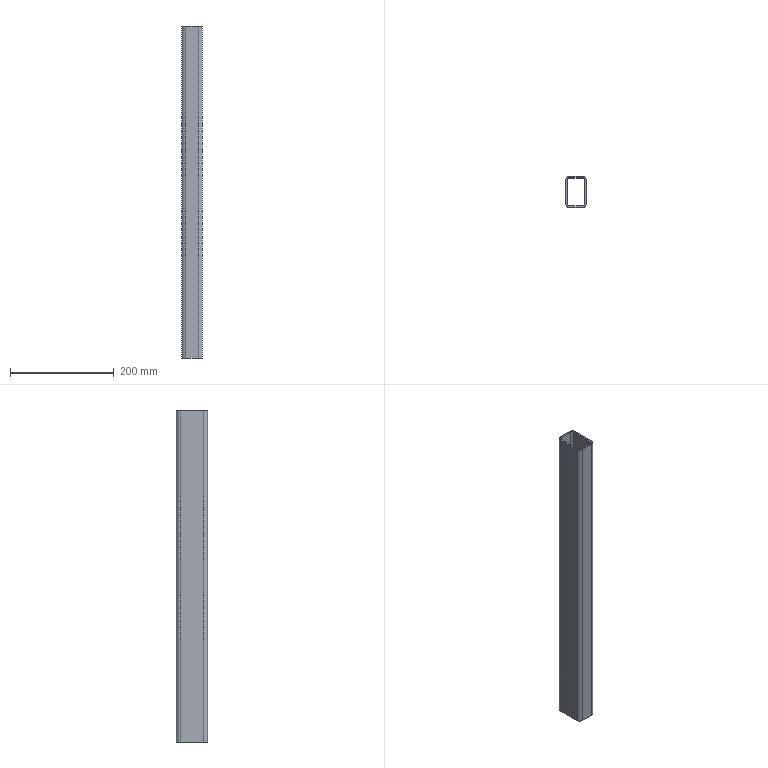Part | SolidWorks | features BaseBody 1 | 1 solid | 18 faces | box 40 x 60 x 640 mm | volume 341182 mm3 | plane 10 | cylinder 8 | commonest cylinder face diameters 9 x4 15 x4
STEP:
#1=CARTESIAN_POINT('',(17.,22.5,30.));
#2=VERTEX_POINT('',#1);
#3=CARTESIAN_POINT('',(17.,22.5,670.));
#4=VERTEX_POINT('',#3);
#5=CARTESIAN_POINT('',(17.,22.5,0.));
#6=DIRECTION('',(0.,0.,1.));
#7=VECTOR('',#6,1000.);
#8=LINE('',#5,#7);
#9=EDGE_CURVE('',#2,#4,#8,.T.);
#10=ORIENTED_EDGE('',*,*,#9,.F.);
#11=CARTESIAN_POINT('',(17.,-22.5,30.));
#12=VERTEX_POINT('',#11);
#13=CARTESIAN_POINT('',(17.,22.5,30.));
#14=DIRECTION('',(0.,1.,0.));
#15=VECTOR('',#14,1000.);
#16=LINE('',#13,#15);
#17=EDGE_CURVE('',#12,#2,#16,.T.);
#18=ORIENTED_EDGE('',*,*,#17,.F.);
#19=CARTESIAN_POINT('',(17.,-22.5,670.));
#20=VERTEX_POINT('',#19);
#21=CARTESIAN_POINT('',(17.,-22.5,0.));
#22=DIRECTION('',(0.,0.,-1.));
#23=VECTOR('',#22,1000.);
#24=LINE('',#21,#23);
#25=EDGE_CURVE('',#20,#12,#24,.T.);
#26=ORIENTED_EDGE('',*,*,#25,.F.);
#27=CARTESIAN_POINT('',(17.,22.5,670.));
#28=DIRECTION('',(0.,-1.,0.));
#29=VECTOR('',#28,1000.);
#30=LINE('',#27,#29);
#31=EDGE_CURVE('',#4,#20,#30,.T.);
#32=ORIENTED_EDGE('',*,*,#31,.F.);
#33=EDGE_LOOP('',(#10,#18,#26,#32));
#34=FACE_OUTER_BOUND('',#33,.T.);
#35=CARTESIAN_POINT('',(17.,22.5,0.));
#36=DIRECTION('',(1.,0.,0.));
#37=DIRECTION('',(0.,1.,0.));
#38=AXIS2_PLACEMENT_3D('',#35,#36,#37);
#39=PLANE('',#38);
#40=ADVANCED_FACE('',(#34),#39,.F.);
#41=CARTESIAN_POINT('',(-17.,-22.5,670.));
#42=VERTEX_POINT('',#41);
#43=CARTESIAN_POINT('',(-17.,22.5,670.));
#44=VERTEX_POINT('',#43);
#45=CARTESIAN_POINT('',(-17.,0.,670.));
#46=DIRECTION('',(0.,1.,0.));
#47=VECTOR('',#46,1000.);
#48=LINE('',#45,#47);
#49=EDGE_CURVE('',#42,#44,#48,.T.);
#50=ORIENTED_EDGE('',*,*,#49,.T.);
#51=CARTESIAN_POINT('',(-12.5,27.,670.));
#52=VERTEX_POINT('',#51);
#53=CARTESIAN_POINT('',(-12.5,22.5,670.));
#54=DIRECTION('',(0.,0.,-1.));
#55=DIRECTION('',(1.,0.,0.));
#56=AXIS2_PLACEMENT_3D('',#53,#54,#55);
#57=CIRCLE('',#56,4.5);
#58=EDGE_CURVE('',#44,#52,#57,.T.);
#59=ORIENTED_EDGE('',*,*,#58,.T.);
#60=CARTESIAN_POINT('',(12.5,27.,670.));
#61=VERTEX_POINT('',#60);
#62=CARTESIAN_POINT('',(0.,27.,670.));
#63=DIRECTION('',(1.,0.,0.));
#64=VECTOR('',#63,1000.);
#65=LINE('',#62,#64);
#66=EDGE_CURVE('',#52,#61,#65,.T.);
#67=ORIENTED_EDGE('',*,*,#66,.T.);
#68=CARTESIAN_POINT('',(12.5,22.5,670.));
#69=DIRECTION('',(0.,0.,-1.));
#70=DIRECTION('',(1.,0.,0.));
#71=AXIS2_PLACEMENT_3D('',#68,#69,#70);
#72=CIRCLE('',#71,4.5);
#73=EDGE_CURVE('',#61,#4,#72,.T.);
#74=ORIENTED_EDGE('',*,*,#73,.T.);
#75=ORIENTED_EDGE('',*,*,#31,.T.);
#76=CARTESIAN_POINT('',(12.5,-27.,670.));
#77=VERTEX_POINT('',#76);
#78=CARTESIAN_POINT('',(12.5,-22.5,670.));
#79=DIRECTION('',(0.,0.,-1.));
#80=DIRECTION('',(1.,0.,0.));
#81=AXIS2_PLACEMENT_3D('',#78,#79,#80);
#82=CIRCLE('',#81,4.5);
#83=EDGE_CURVE('',#20,#77,#82,.T.);
#84=ORIENTED_EDGE('',*,*,#83,.T.);
#85=CARTESIAN_POINT('',(-12.5,-27.,670.));
#86=VERTEX_POINT('',#85);
#87=CARTESIAN_POINT('',(0.,-27.,670.));
#88=DIRECTION('',(-1.,0.,0.));
#89=VECTOR('',#88,1000.);
#90=LINE('',#87,#89);
#91=EDGE_CURVE('',#77,#86,#90,.T.);
#92=ORIENTED_EDGE('',*,*,#91,.T.);
#93=CARTESIAN_POINT('',(-12.5,-22.5,670.));
#94=DIRECTION('',(0.,0.,-1.));
#95=DIRECTION('',(1.,0.,0.));
#96=AXIS2_PLACEMENT_3D('',#93,#94,#95);
#97=CIRCLE('',#96,4.5);
#98=EDGE_CURVE('',#86,#42,#97,.T.);
#99=ORIENTED_EDGE('',*,*,#98,.T.);
#100=EDGE_LOOP('',(#50,#59,#67,#74,#75,#84,#92,#99));
#101=FACE_BOUND('',#100,.T.);
#102=CARTESIAN_POINT('',(12.5,30.,670.));
#103=VERTEX_POINT('',#102);
#104=CARTESIAN_POINT('',(-12.5,30.,670.));
#105=VERTEX_POINT('',#104);
#106=CARTESIAN_POINT('',(0.,30.,670.));
#107=DIRECTION('',(-1.,0.,0.));
#108=VECTOR('',#107,1000.);
#109=LINE('',#106,#108);
#110=EDGE_CURVE('',#103,#105,#109,.T.);
#111=ORIENTED_EDGE('',*,*,#110,.T.);
#112=CARTESIAN_POINT('',(-20.,22.5,670.));
#113=VERTEX_POINT('',#112);
#114=CARTESIAN_POINT('',(-12.5,22.5,670.));
#115=DIRECTION('',(0.,0.,1.));
#116=DIRECTION('',(1.,0.,0.));
#117=AXIS2_PLACEMENT_3D('',#114,#115,#116);
#118=CIRCLE('',#117,7.5);
#119=EDGE_CURVE('',#105,#113,#118,.T.);
#120=ORIENTED_EDGE('',*,*,#119,.T.);
#121=CARTESIAN_POINT('',(-20.,-22.5,670.));
#122=VERTEX_POINT('',#121);
#123=CARTESIAN_POINT('',(-20.,0.,670.));
#124=DIRECTION('',(0.,-1.,0.));
#125=VECTOR('',#124,1000.);
#126=LINE('',#123,#125);
#127=EDGE_CURVE('',#113,#122,#126,.T.);
#128=ORIENTED_EDGE('',*,*,#127,.T.);
#129=CARTESIAN_POINT('',(-12.5,-30.,670.));
#130=VERTEX_POINT('',#129);
#131=CARTESIAN_POINT('',(-12.5,-22.5,670.));
#132=DIRECTION('',(0.,0.,1.));
#133=DIRECTION('',(1.,0.,0.));
#134=AXIS2_PLACEMENT_3D('',#131,#132,#133);
#135=CIRCLE('',#134,7.5);
#136=EDGE_CURVE('',#122,#130,#135,.T.);
#137=ORIENTED_EDGE('',*,*,#136,.T.);
#138=CARTESIAN_POINT('',(12.5,-30.,670.));
#139=VERTEX_POINT('',#138);
#140=CARTESIAN_POINT('',(0.,-30.,670.));
#141=DIRECTION('',(1.,0.,0.));
#142=VECTOR('',#141,1000.);
#143=LINE('',#140,#142);
#144=EDGE_CURVE('',#130,#139,#143,.T.);
#145=ORIENTED_EDGE('',*,*,#144,.T.);
#146=CARTESIAN_POINT('',(20.,-22.5,670.));
#147=VERTEX_POINT('',#146);
#148=CARTESIAN_POINT('',(12.5,-22.5,670.));
#149=DIRECTION('',(0.,0.,1.));
#150=DIRECTION('',(1.,0.,0.));
#151=AXIS2_PLACEMENT_3D('',#148,#149,#150);
#152=CIRCLE('',#151,7.5);
#153=EDGE_CURVE('',#139,#147,#152,.T.);
#154=ORIENTED_EDGE('',*,*,#153,.T.);
#155=CARTESIAN_POINT('',(20.,22.5,670.));
#156=VERTEX_POINT('',#155);
#157=CARTESIAN_POINT('',(20.,0.,670.));
#158=DIRECTION('',(0.,1.,0.));
#159=VECTOR('',#158,1000.);
#160=LINE('',#157,#159);
#161=EDGE_CURVE('',#147,#156,#160,.T.);
#162=ORIENTED_EDGE('',*,*,#161,.T.);
#163=CARTESIAN_POINT('',(12.5,22.5,670.));
#164=DIRECTION('',(0.,0.,1.));
#165=DIRECTION('',(1.,0.,0.));
#166=AXIS2_PLACEMENT_3D('',#163,#164,#165);
#167=CIRCLE('',#166,7.5);
#168=EDGE_CURVE('',#156,#103,#167,.T.);
#169=ORIENTED_EDGE('',*,*,#168,.T.);
#170=EDGE_LOOP('',(#111,#120,#128,#137,#145,#154,#162,#169));
#171=FACE_OUTER_BOUND('',#170,.T.);
#172=CARTESIAN_POINT('',(0.,0.,670.));
#173=DIRECTION('',(0.,0.,1.));
#174=DIRECTION('',(1.,0.,0.));
#175=AXIS2_PLACEMENT_3D('',#172,#173,#174);
#176=PLANE('',#175);
#177=ADVANCED_FACE('',(#101,#171),#176,.T.);
#178=CARTESIAN_POINT('',(12.5,27.,30.));
#179=VERTEX_POINT('',#178);
#180=CARTESIAN_POINT('',(12.5,27.,0.));
#181=DIRECTION('',(0.,0.,1.));
#182=VECTOR('',#181,1000.);
#183=LINE('',#180,#182);
#184=EDGE_CURVE('',#179,#61,#183,.T.);
#185=ORIENTED_EDGE('',*,*,#184,.F.);
#186=CARTESIAN_POINT('',(12.5,22.5,30.));
#187=DIRECTION('',(0.,0.,1.));
#188=DIRECTION('',(1.,0.,0.));
#189=AXIS2_PLACEMENT_3D('',#186,#187,#188);
#190=CIRCLE('',#189,4.5);
#191=EDGE_CURVE('',#2,#179,#190,.T.);
#192=ORIENTED_EDGE('',*,*,#191,.F.);
#193=ORIENTED_EDGE('',*,*,#9,.T.);
#194=ORIENTED_EDGE('',*,*,#73,.F.);
#195=EDGE_LOOP('',(#185,#192,#193,#194));
#196=FACE_OUTER_BOUND('',#195,.T.);
#197=CARTESIAN_POINT('',(12.5,22.5,0.));
#198=DIRECTION('',(0.,0.,1.));
#199=DIRECTION('',(1.,0.,0.));
#200=AXIS2_PLACEMENT_3D('',#197,#198,#199);
#201=CYLINDRICAL_SURFACE('',#200,4.5);
#202=ADVANCED_FACE('',(#196),#201,.F.);
#203=CARTESIAN_POINT('',(-17.,22.5,30.));
#204=VERTEX_POINT('',#203);
#205=CARTESIAN_POINT('',(-12.5,27.,30.));
#206=VERTEX_POINT('',#205);
#207=CARTESIAN_POINT('',(-12.5,22.5,30.));
#208=DIRECTION('',(0.,0.,-1.));
#209=DIRECTION('',(1.,0.,0.));
#210=AXIS2_PLACEMENT_3D('',#207,#208,#209);
#211=CIRCLE('',#210,4.5);
#212=EDGE_CURVE('',#204,#206,#211,.T.);
#213=ORIENTED_EDGE('',*,*,#212,.F.);
#214=CARTESIAN_POINT('',(-17.,-22.5,30.));
#215=VERTEX_POINT('',#214);
#216=CARTESIAN_POINT('',(-17.,0.,30.));
#217=DIRECTION('',(0.,1.,0.));
#218=VECTOR('',#217,1000.);
#219=LINE('',#216,#218);
#220=EDGE_CURVE('',#215,#204,#219,.T.);
#221=ORIENTED_EDGE('',*,*,#220,.F.);
#222=CARTESIAN_POINT('',(-12.5,-27.,30.));
#223=VERTEX_POINT('',#222);
#224=CARTESIAN_POINT('',(-12.5,-22.5,30.));
#225=DIRECTION('',(0.,0.,-1.));
#226=DIRECTION('',(1.,0.,0.));
#227=AXIS2_PLACEMENT_3D('',#224,#225,#226);
#228=CIRCLE('',#227,4.5);
#229=EDGE_CURVE('',#223,#215,#228,.T.);
#230=ORIENTED_EDGE('',*,*,#229,.F.);
#231=CARTESIAN_POINT('',(12.5,-27.,30.));
#232=VERTEX_POINT('',#231);
#233=CARTESIAN_POINT('',(0.,-27.,30.));
#234=DIRECTION('',(-1.,0.,0.));
#235=VECTOR('',#234,1000.);
#236=LINE('',#233,#235);
#237=EDGE_CURVE('',#232,#223,#236,.T.);
#238=ORIENTED_EDGE('',*,*,#237,.F.);
#239=CARTESIAN_POINT('',(12.5,-22.5,30.));
#240=DIRECTION('',(0.,0.,-1.));
#241=DIRECTION('',(1.,0.,0.));
#242=AXIS2_PLACEMENT_3D('',#239,#240,#241);
#243=CIRCLE('',#242,4.5);
#244=EDGE_CURVE('',#12,#232,#243,.T.);
#245=ORIENTED_EDGE('',*,*,#244,.F.);
#246=ORIENTED_EDGE('',*,*,#17,.T.);
#247=ORIENTED_EDGE('',*,*,#191,.T.);
#248=CARTESIAN_POINT('',(0.,27.,30.));
#249=DIRECTION('',(1.,0.,0.));
#250=VECTOR('',#249,1000.);
#251=LINE('',#248,#250);
#252=EDGE_CURVE('',#206,#179,#251,.T.);
#253=ORIENTED_EDGE('',*,*,#252,.F.);
#254=EDGE_LOOP('',(#213,#221,#230,#238,#245,#246,#247,#253));
#255=FACE_BOUND('',#254,.T.);
#256=CARTESIAN_POINT('',(-12.5,30.,30.));
#257=VERTEX_POINT('',#256);
#258=CARTESIAN_POINT('',(-20.,22.5,30.));
#259=VERTEX_POINT('',#258);
#260=CARTESIAN_POINT('',(-12.5,22.5,30.));
#261=DIRECTION('',(0.,0.,1.));
#262=DIRECTION('',(1.,0.,0.));
#263=AXIS2_PLACEMENT_3D('',#260,#261,#262);
#264=CIRCLE('',#263,7.5);
#265=EDGE_CURVE('',#257,#259,#264,.T.);
#266=ORIENTED_EDGE('',*,*,#265,.F.);
#267=CARTESIAN_POINT('',(12.5,30.,30.));
#268=VERTEX_POINT('',#267);
#269=CARTESIAN_POINT('',(0.,30.,30.));
#270=DIRECTION('',(-1.,0.,0.));
#271=VECTOR('',#270,1000.);
#272=LINE('',#269,#271);
#273=EDGE_CURVE('',#268,#257,#272,.T.);
#274=ORIENTED_EDGE('',*,*,#273,.F.);
#275=CARTESIAN_POINT('',(20.,22.5,30.));
#276=VERTEX_POINT('',#275);
#277=CARTESIAN_POINT('',(12.5,22.5,30.));
#278=DIRECTION('',(0.,0.,1.));
#279=DIRECTION('',(1.,0.,0.));
#280=AXIS2_PLACEMENT_3D('',#277,#278,#279);
#281=CIRCLE('',#280,7.5);
#282=EDGE_CURVE('',#276,#268,#281,.T.);
#283=ORIENTED_EDGE('',*,*,#282,.F.);
#284=CARTESIAN_POINT('',(20.,-22.5,30.));
#285=VERTEX_POINT('',#284);
#286=CARTESIAN_POINT('',(20.,0.,30.));
#287=DIRECTION('',(0.,1.,0.));
#288=VECTOR('',#287,1000.);
#289=LINE('',#286,#288);
#290=EDGE_CURVE('',#285,#276,#289,.T.);
#291=ORIENTED_EDGE('',*,*,#290,.F.);
#292=CARTESIAN_POINT('',(12.5,-30.,30.));
#293=VERTEX_POINT('',#292);
#294=CARTESIAN_POINT('',(12.5,-22.5,30.));
#295=DIRECTION('',(0.,0.,1.));
#296=DIRECTION('',(1.,0.,0.));
#297=AXIS2_PLACEMENT_3D('',#294,#295,#296);
#298=CIRCLE('',#297,7.5);
#299=EDGE_CURVE('',#293,#285,#298,.T.);
#300=ORIENTED_EDGE('',*,*,#299,.F.);
#301=CARTESIAN_POINT('',(-12.5,-30.,30.));
#302=VERTEX_POINT('',#301);
#303=CARTESIAN_POINT('',(0.,-30.,30.));
#304=DIRECTION('',(1.,0.,0.));
#305=VECTOR('',#304,1000.);
#306=LINE('',#303,#305);
#307=EDGE_CURVE('',#302,#293,#306,.T.);
#308=ORIENTED_EDGE('',*,*,#307,.F.);
#309=CARTESIAN_POINT('',(-20.,-22.5,30.));
#310=VERTEX_POINT('',#309);
#311=CARTESIAN_POINT('',(-12.5,-22.5,30.));
#312=DIRECTION('',(0.,0.,1.));
#313=DIRECTION('',(1.,0.,0.));
#314=AXIS2_PLACEMENT_3D('',#311,#312,#313);
#315=CIRCLE('',#314,7.5);
#316=EDGE_CURVE('',#310,#302,#315,.T.);
#317=ORIENTED_EDGE('',*,*,#316,.F.);
#318=CARTESIAN_POINT('',(-20.,0.,30.));
#319=DIRECTION('',(0.,-1.,0.));
#320=VECTOR('',#319,1000.);
#321=LINE('',#318,#320);
#322=EDGE_CURVE('',#259,#310,#321,.T.);
#323=ORIENTED_EDGE('',*,*,#322,.F.);
#324=EDGE_LOOP('',(#266,#274,#283,#291,#300,#308,#317,#323));
#325=FACE_OUTER_BOUND('',#324,.T.);
#326=CARTESIAN_POINT('',(0.,0.,30.));
#327=DIRECTION('',(0.,0.,1.));
#328=DIRECTION('',(1.,0.,0.));
#329=AXIS2_PLACEMENT_3D('',#326,#327,#328);
#330=PLANE('',#329);
#331=ADVANCED_FACE('',(#255,#325),#330,.F.);
#332=ORIENTED_EDGE('',*,*,#25,.T.);
#333=ORIENTED_EDGE('',*,*,#244,.T.);
#334=CARTESIAN_POINT('',(12.5,-27.,0.));
#335=DIRECTION('',(0.,0.,-1.));
#336=VECTOR('',#335,1000.);
#337=LINE('',#334,#336);
#338=EDGE_CURVE('',#77,#232,#337,.T.);
#339=ORIENTED_EDGE('',*,*,#338,.F.);
#340=ORIENTED_EDGE('',*,*,#83,.F.);
#341=EDGE_LOOP('',(#332,#333,#339,#340));
#342=FACE_OUTER_BOUND('',#341,.T.);
#343=CARTESIAN_POINT('',(12.5,-22.5,0.));
#344=DIRECTION('',(0.,0.,1.));
#345=DIRECTION('',(1.,0.,0.));
#346=AXIS2_PLACEMENT_3D('',#343,#344,#345);
#347=CYLINDRICAL_SURFACE('',#346,4.5);
#348=ADVANCED_FACE('',(#342),#347,.F.);
#349=CARTESIAN_POINT('',(-17.,22.5,0.));
#350=DIRECTION('',(0.,0.,1.));
#351=VECTOR('',#350,1000.);
#352=LINE('',#349,#351);
#353=EDGE_CURVE('',#204,#44,#352,.T.);
#354=ORIENTED_EDGE('',*,*,#353,.F.);
#355=ORIENTED_EDGE('',*,*,#212,.T.);
#356=CARTESIAN_POINT('',(-12.5,27.,0.));
#357=DIRECTION('',(0.,0.,-1.));
#358=VECTOR('',#357,1000.);
#359=LINE('',#356,#358);
#360=EDGE_CURVE('',#52,#206,#359,.T.);
#361=ORIENTED_EDGE('',*,*,#360,.F.);
#362=ORIENTED_EDGE('',*,*,#58,.F.);
#363=EDGE_LOOP('',(#354,#355,#361,#362));
#364=FACE_OUTER_BOUND('',#363,.T.);
#365=CARTESIAN_POINT('',(-12.5,22.5,0.));
#366=DIRECTION('',(0.,0.,1.));
#367=DIRECTION('',(1.,0.,0.));
#368=AXIS2_PLACEMENT_3D('',#365,#366,#367);
#369=CYLINDRICAL_SURFACE('',#368,4.5);
#370=ADVANCED_FACE('',(#364),#369,.F.);
#371=CARTESIAN_POINT('',(-17.,-22.5,0.));
#372=DIRECTION('',(0.,0.,1.));
#373=VECTOR('',#372,1000.);
#374=LINE('',#371,#373);
#375=EDGE_CURVE('',#215,#42,#374,.T.);
#376=ORIENTED_EDGE('',*,*,#375,.F.);
#377=ORIENTED_EDGE('',*,*,#220,.T.);
#378=ORIENTED_EDGE('',*,*,#353,.T.);
#379=ORIENTED_EDGE('',*,*,#49,.F.);
#380=EDGE_LOOP('',(#376,#377,#378,#379));
#381=FACE_OUTER_BOUND('',#380,.T.);
#382=CARTESIAN_POINT('',(-17.,-22.5,0.));
#383=DIRECTION('',(-1.,0.,0.));
#384=DIRECTION('',(0.,-1.,0.));
#385=AXIS2_PLACEMENT_3D('',#382,#383,#384);
#386=PLANE('',#385);
#387=ADVANCED_FACE('',(#381),#386,.F.);
#388=CARTESIAN_POINT('',(-12.5,-27.,0.));
#389=DIRECTION('',(0.,0.,1.));
#390=VECTOR('',#389,1000.);
#391=LINE('',#388,#390);
#392=EDGE_CURVE('',#223,#86,#391,.T.);
#393=ORIENTED_EDGE('',*,*,#392,.F.);
#394=ORIENTED_EDGE('',*,*,#229,.T.);
#395=ORIENTED_EDGE('',*,*,#375,.T.);
#396=ORIENTED_EDGE('',*,*,#98,.F.);
#397=EDGE_LOOP('',(#393,#394,#395,#396));
#398=FACE_OUTER_BOUND('',#397,.T.);
#399=CARTESIAN_POINT('',(-12.5,-22.5,0.));
#400=DIRECTION('',(0.,0.,1.));
#401=DIRECTION('',(1.,0.,0.));
#402=AXIS2_PLACEMENT_3D('',#399,#400,#401);
#403=CYLINDRICAL_SURFACE('',#402,4.5);
#404=ADVANCED_FACE('',(#398),#403,.F.);
#405=ORIENTED_EDGE('',*,*,#338,.T.);
#406=ORIENTED_EDGE('',*,*,#237,.T.);
#407=ORIENTED_EDGE('',*,*,#392,.T.);
#408=ORIENTED_EDGE('',*,*,#91,.F.);
#409=EDGE_LOOP('',(#405,#406,#407,#408));
#410=FACE_OUTER_BOUND('',#409,.T.);
#411=CARTESIAN_POINT('',(12.5,-27.,0.));
#412=DIRECTION('',(0.,-1.,0.));
#413=DIRECTION('',(1.,0.,0.));
#414=AXIS2_PLACEMENT_3D('',#411,#412,#413);
#415=PLANE('',#414);
#416=ADVANCED_FACE('',(#410),#415,.F.);
#417=ORIENTED_EDGE('',*,*,#360,.T.);
#418=ORIENTED_EDGE('',*,*,#252,.T.);
#419=ORIENTED_EDGE('',*,*,#184,.T.);
#420=ORIENTED_EDGE('',*,*,#66,.F.);
#421=EDGE_LOOP('',(#417,#418,#419,#420));
#422=FACE_OUTER_BOUND('',#421,.T.);
#423=CARTESIAN_POINT('',(-12.5,27.,0.));
#424=DIRECTION('',(0.,1.,0.));
#425=DIRECTION('',(-1.,0.,0.));
#426=AXIS2_PLACEMENT_3D('',#423,#424,#425);
#427=PLANE('',#426);
#428=ADVANCED_FACE('',(#422),#427,.F.);
#429=ORIENTED_EDGE('',*,*,#265,.T.);
#430=CARTESIAN_POINT('',(-20.,22.5,0.));
#431=DIRECTION('',(0.,0.,1.));
#432=VECTOR('',#431,1000.);
#433=LINE('',#430,#432);
#434=EDGE_CURVE('',#259,#113,#433,.T.);
#435=ORIENTED_EDGE('',*,*,#434,.T.);
#436=ORIENTED_EDGE('',*,*,#119,.F.);
#437=CARTESIAN_POINT('',(-12.5,30.,0.));
#438=DIRECTION('',(0.,0.,-1.));
#439=VECTOR('',#438,1000.);
#440=LINE('',#437,#439);
#441=EDGE_CURVE('',#105,#257,#440,.T.);
#442=ORIENTED_EDGE('',*,*,#441,.T.);
#443=EDGE_LOOP('',(#429,#435,#436,#442));
#444=FACE_OUTER_BOUND('',#443,.T.);
#445=CARTESIAN_POINT('',(-12.5,22.5,0.));
#446=DIRECTION('',(0.,0.,1.));
#447=DIRECTION('',(1.,0.,0.));
#448=AXIS2_PLACEMENT_3D('',#445,#446,#447);
#449=CYLINDRICAL_SURFACE('',#448,7.5);
#450=ADVANCED_FACE('',(#444),#449,.T.);
#451=ORIENTED_EDGE('',*,*,#273,.T.);
#452=ORIENTED_EDGE('',*,*,#441,.F.);
#453=ORIENTED_EDGE('',*,*,#110,.F.);
#454=CARTESIAN_POINT('',(12.5,30.,0.));
#455=DIRECTION('',(0.,0.,-1.));
#456=VECTOR('',#455,1000.);
#457=LINE('',#454,#456);
#458=EDGE_CURVE('',#103,#268,#457,.T.);
#459=ORIENTED_EDGE('',*,*,#458,.T.);
#460=EDGE_LOOP('',(#451,#452,#453,#459));
#461=FACE_OUTER_BOUND('',#460,.T.);
#462=CARTESIAN_POINT('',(-12.5,30.,0.));
#463=DIRECTION('',(0.,1.,0.));
#464=DIRECTION('',(0.,0.,1.));
#465=AXIS2_PLACEMENT_3D('',#462,#463,#464);
#466=PLANE('',#465);
#467=ADVANCED_FACE('',(#461),#466,.T.);
#468=ORIENTED_EDGE('',*,*,#282,.T.);
#469=ORIENTED_EDGE('',*,*,#458,.F.);
#470=ORIENTED_EDGE('',*,*,#168,.F.);
#471=CARTESIAN_POINT('',(20.,22.5,0.));
#472=DIRECTION('',(0.,0.,-1.));
#473=VECTOR('',#472,1000.);
#474=LINE('',#471,#473);
#475=EDGE_CURVE('',#156,#276,#474,.T.);
#476=ORIENTED_EDGE('',*,*,#475,.T.);
#477=EDGE_LOOP('',(#468,#469,#470,#476));
#478=FACE_OUTER_BOUND('',#477,.T.);
#479=CARTESIAN_POINT('',(12.5,22.5,0.));
#480=DIRECTION('',(0.,0.,1.));
#481=DIRECTION('',(1.,0.,0.));
#482=AXIS2_PLACEMENT_3D('',#479,#480,#481);
#483=CYLINDRICAL_SURFACE('',#482,7.5);
#484=ADVANCED_FACE('',(#478),#483,.T.);
#485=ORIENTED_EDGE('',*,*,#290,.T.);
#486=ORIENTED_EDGE('',*,*,#475,.F.);
#487=ORIENTED_EDGE('',*,*,#161,.F.);
#488=CARTESIAN_POINT('',(20.,-22.5,0.));
#489=DIRECTION('',(0.,0.,-1.));
#490=VECTOR('',#489,1000.);
#491=LINE('',#488,#490);
#492=EDGE_CURVE('',#147,#285,#491,.T.);
#493=ORIENTED_EDGE('',*,*,#492,.T.);
#494=EDGE_LOOP('',(#485,#486,#487,#493));
#495=FACE_OUTER_BOUND('',#494,.T.);
#496=CARTESIAN_POINT('',(20.,22.5,0.));
#497=DIRECTION('',(1.,0.,0.));
#498=DIRECTION('',(0.,0.,-1.));
#499=AXIS2_PLACEMENT_3D('',#496,#497,#498);
#500=PLANE('',#499);
#501=ADVANCED_FACE('',(#495),#500,.T.);
#502=ORIENTED_EDGE('',*,*,#299,.T.);
#503=ORIENTED_EDGE('',*,*,#492,.F.);
#504=ORIENTED_EDGE('',*,*,#153,.F.);
#505=CARTESIAN_POINT('',(12.5,-30.,0.));
#506=DIRECTION('',(0.,0.,-1.));
#507=VECTOR('',#506,1000.);
#508=LINE('',#505,#507);
#509=EDGE_CURVE('',#139,#293,#508,.T.);
#510=ORIENTED_EDGE('',*,*,#509,.T.);
#511=EDGE_LOOP('',(#502,#503,#504,#510));
#512=FACE_OUTER_BOUND('',#511,.T.);
#513=CARTESIAN_POINT('',(12.5,-22.5,0.));
#514=DIRECTION('',(0.,0.,1.));
#515=DIRECTION('',(1.,0.,0.));
#516=AXIS2_PLACEMENT_3D('',#513,#514,#515);
#517=CYLINDRICAL_SURFACE('',#516,7.5);
#518=ADVANCED_FACE('',(#512),#517,.T.);
#519=ORIENTED_EDGE('',*,*,#307,.T.);
#520=ORIENTED_EDGE('',*,*,#509,.F.);
#521=ORIENTED_EDGE('',*,*,#144,.F.);
#522=CARTESIAN_POINT('',(-12.5,-30.,0.));
#523=DIRECTION('',(0.,0.,-1.));
#524=VECTOR('',#523,1000.);
#525=LINE('',#522,#524);
#526=EDGE_CURVE('',#130,#302,#525,.T.);
#527=ORIENTED_EDGE('',*,*,#526,.T.);
#528=EDGE_LOOP('',(#519,#520,#521,#527));
#529=FACE_OUTER_BOUND('',#528,.T.);
#530=CARTESIAN_POINT('',(12.5,-30.,0.));
#531=DIRECTION('',(0.,-1.,0.));
#532=DIRECTION('',(1.,0.,0.));
#533=AXIS2_PLACEMENT_3D('',#530,#531,#532);
#534=PLANE('',#533);
#535=ADVANCED_FACE('',(#529),#534,.T.);
#536=ORIENTED_EDGE('',*,*,#316,.T.);
#537=ORIENTED_EDGE('',*,*,#526,.F.);
#538=ORIENTED_EDGE('',*,*,#136,.F.);
#539=CARTESIAN_POINT('',(-20.,-22.5,0.));
#540=DIRECTION('',(0.,0.,-1.));
#541=VECTOR('',#540,1000.);
#542=LINE('',#539,#541);
#543=EDGE_CURVE('',#122,#310,#542,.T.);
#544=ORIENTED_EDGE('',*,*,#543,.T.);
#545=EDGE_LOOP('',(#536,#537,#538,#544));
#546=FACE_OUTER_BOUND('',#545,.T.);
#547=CARTESIAN_POINT('',(-12.5,-22.5,0.));
#548=DIRECTION('',(0.,0.,1.));
#549=DIRECTION('',(1.,0.,0.));
#550=AXIS2_PLACEMENT_3D('',#547,#548,#549);
#551=CYLINDRICAL_SURFACE('',#550,7.5);
#552=ADVANCED_FACE('',(#546),#551,.T.);
#553=ORIENTED_EDGE('',*,*,#322,.T.);
#554=ORIENTED_EDGE('',*,*,#543,.F.);
#555=ORIENTED_EDGE('',*,*,#127,.F.);
#556=ORIENTED_EDGE('',*,*,#434,.F.);
#557=EDGE_LOOP('',(#553,#554,#555,#556));
#558=FACE_OUTER_BOUND('',#557,.T.);
#559=CARTESIAN_POINT('',(-20.,-22.5,0.));
#560=DIRECTION('',(-1.,0.,0.));
#561=DIRECTION('',(0.,-1.,0.));
#562=AXIS2_PLACEMENT_3D('',#559,#560,#561);
#563=PLANE('',#562);
#564=ADVANCED_FACE('',(#558),#563,.T.);
#565=CLOSED_SHELL('',(#40,#177,#202,#331,#348,#370,#387,#404,#416,#428,#450,#467,#484,#501,#518,#535,#552,#564));
#566=MANIFOLD_SOLID_BREP('',#565);
#567=CARTESIAN_POINT('',(0.,0.,0.));
#568=DIRECTION('',(0.,0.,1.));
#569=DIRECTION('',(1.,0.,0.));
#570=AXIS2_PLACEMENT_3D('',#567,#568,#569);
#571=(LENGTH_UNIT()NAMED_UNIT(*)SI_UNIT(.MILLI.,.METRE.));
#572=UNCERTAINTY_MEASURE_WITH_UNIT(LENGTH_MEASURE(0.00001),#571,'','');
#573=(NAMED_UNIT(*)PLANE_ANGLE_UNIT()SI_UNIT($,.RADIAN.));
#574=(NAMED_UNIT(*)SI_UNIT($,.STERADIAN.)SOLID_ANGLE_UNIT());
#575=(GEOMETRIC_REPRESENTATION_CONTEXT(3)GLOBAL_UNCERTAINTY_ASSIGNED_CONTEXT((#572))GLOBAL_UNIT_ASSIGNED_CONTEXT((#571,#573,#574))REPRESENTATION_CONTEXT('',''));
#576=ADVANCED_BREP_SHAPE_REPRESENTATION('',(#566,#570),#575);